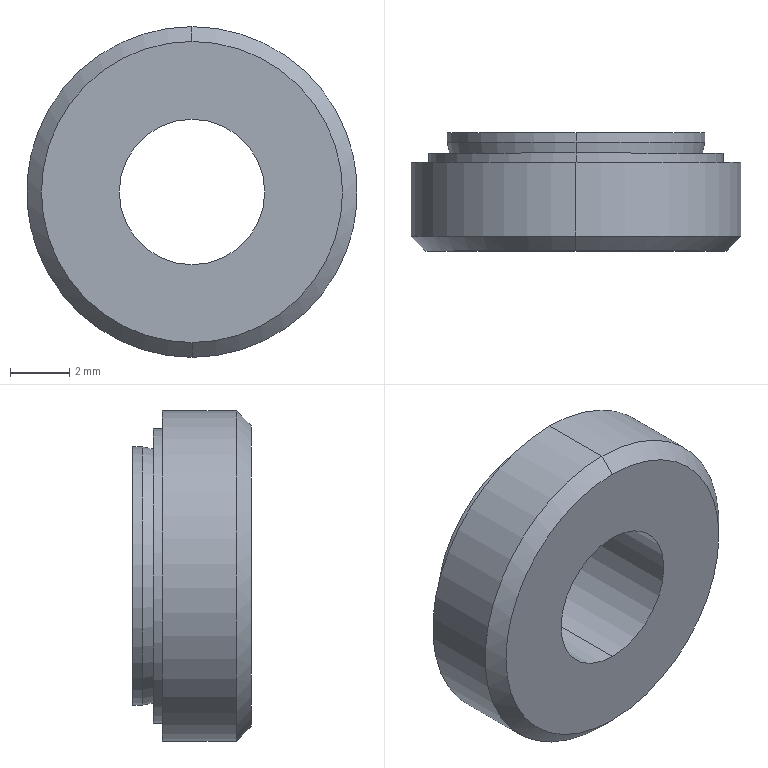Part | NX | features solid 2 | 1 solid | 18 faces | box 11.18 x 4 x 11.18 mm | volume 276.924 mm3 | cylinder 8 | cone 6 | plane 4 | commonest cylinder face diameters 4.917 x2 8.73 x2 9.955 x2 11.18 x2
STEP:
#1=CARTESIAN_POINT('',(-24.5,-9.,-1048.59));
#2=VERTEX_POINT('',#1);
#3=CARTESIAN_POINT('',(-24.5,-6.5,-1048.59));
#4=VERTEX_POINT('',#3);
#5=CARTESIAN_POINT('',(-24.5,-9.,-1048.59));
#6=DIRECTION('',(0.,1.,0.));
#7=VECTOR('',#6,1000.);
#8=LINE('',#5,#7);
#9=EDGE_CURVE('',#2,#4,#8,.T.);
#10=ORIENTED_EDGE('',*,*,#9,.T.);
#11=CARTESIAN_POINT('',(-24.5,-6.5,-1037.41));
#12=VERTEX_POINT('',#11);
#13=CARTESIAN_POINT('',(-24.5,-6.5,-1043.));
#14=DIRECTION('',(0.,-1.,0.));
#15=DIRECTION('',(0.,0.,-1.));
#16=AXIS2_PLACEMENT_3D('',#13,#14,#15);
#17=CIRCLE('',#16,5.59);
#18=EDGE_CURVE('',#4,#12,#17,.T.);
#19=ORIENTED_EDGE('',*,*,#18,.T.);
#20=CARTESIAN_POINT('',(-24.5,-9.,-1037.41));
#21=VERTEX_POINT('',#20);
#22=CARTESIAN_POINT('',(-24.5,-6.5,-1037.41));
#23=DIRECTION('',(0.,-1.,0.));
#24=VECTOR('',#23,1000.);
#25=LINE('',#22,#24);
#26=EDGE_CURVE('',#12,#21,#25,.T.);
#27=ORIENTED_EDGE('',*,*,#26,.T.);
#28=CARTESIAN_POINT('',(-24.5,-9.,-1043.));
#29=DIRECTION('',(0.,1.,0.));
#30=DIRECTION('',(0.,0.,1.));
#31=AXIS2_PLACEMENT_3D('',#28,#29,#30);
#32=CIRCLE('',#31,5.59);
#33=EDGE_CURVE('',#21,#2,#32,.T.);
#34=ORIENTED_EDGE('',*,*,#33,.T.);
#35=EDGE_LOOP('',(#10,#19,#27,#34));
#36=FACE_BOUND('',#35,.T.);
#37=CARTESIAN_POINT('',(-24.5,-8.752,-1043.));
#38=DIRECTION('',(0.,1.,0.));
#39=DIRECTION('',(0.,0.,1.));
#40=AXIS2_PLACEMENT_3D('',#37,#38,#39);
#41=CYLINDRICAL_SURFACE('',#40,5.59);
#42=ADVANCED_FACE('',(#36),#41,.T.);
#43=CARTESIAN_POINT('',(-24.5,-9.5,-1037.91));
#44=VERTEX_POINT('',#43);
#45=CARTESIAN_POINT('',(-24.5,-9.,-1037.41));
#46=DIRECTION('',(0.,-0.7071,-0.7071));
#47=VECTOR('',#46,1000.);
#48=LINE('',#45,#47);
#49=EDGE_CURVE('',#21,#44,#48,.T.);
#50=ORIENTED_EDGE('',*,*,#49,.T.);
#51=CARTESIAN_POINT('',(-24.5,-9.5,-1048.09));
#52=VERTEX_POINT('',#51);
#53=CARTESIAN_POINT('',(-24.5,-9.5,-1043.));
#54=DIRECTION('',(0.,1.,0.));
#55=DIRECTION('',(0.,0.,1.));
#56=AXIS2_PLACEMENT_3D('',#53,#54,#55);
#57=CIRCLE('',#56,5.09);
#58=EDGE_CURVE('',#44,#52,#57,.T.);
#59=ORIENTED_EDGE('',*,*,#58,.T.);
#60=CARTESIAN_POINT('',(-24.5,-9.,-1048.59));
#61=DIRECTION('',(0.,-0.7071,0.7071));
#62=VECTOR('',#61,1000.);
#63=LINE('',#60,#62);
#64=EDGE_CURVE('',#52,#2,#63,.F.);
#65=ORIENTED_EDGE('',*,*,#64,.T.);
#66=ORIENTED_EDGE('',*,*,#33,.F.);
#67=EDGE_LOOP('',(#50,#59,#65,#66));
#68=FACE_BOUND('',#67,.T.);
#69=CARTESIAN_POINT('',(-24.5,-9.25,-1043.));
#70=DIRECTION('',(0.,1.,0.));
#71=DIRECTION('',(0.,0.,1.));
#72=AXIS2_PLACEMENT_3D('',#69,#70,#71);
#73=CONICAL_SURFACE('',#72,5.34,0.7854);
#74=ADVANCED_FACE('',(#68),#73,.T.);
#75=ORIENTED_EDGE('',*,*,#64,.F.);
#76=CARTESIAN_POINT('',(-24.5,-9.5,-1043.));
#77=DIRECTION('',(0.,1.,0.));
#78=DIRECTION('',(0.,0.,-1.));
#79=AXIS2_PLACEMENT_3D('',#76,#77,#78);
#80=CIRCLE('',#79,5.09);
#81=EDGE_CURVE('',#52,#44,#80,.T.);
#82=ORIENTED_EDGE('',*,*,#81,.T.);
#83=ORIENTED_EDGE('',*,*,#49,.F.);
#84=CARTESIAN_POINT('',(-24.5,-9.,-1043.));
#85=DIRECTION('',(0.,1.,0.));
#86=DIRECTION('',(0.,0.,-1.));
#87=AXIS2_PLACEMENT_3D('',#84,#85,#86);
#88=CIRCLE('',#87,5.59);
#89=EDGE_CURVE('',#2,#21,#88,.T.);
#90=ORIENTED_EDGE('',*,*,#89,.F.);
#91=EDGE_LOOP('',(#75,#82,#83,#90));
#92=FACE_BOUND('',#91,.T.);
#93=CARTESIAN_POINT('',(-24.5,-9.25,-1043.));
#94=DIRECTION('',(0.,1.,0.));
#95=DIRECTION('',(0.,0.,1.));
#96=AXIS2_PLACEMENT_3D('',#93,#94,#95);
#97=CONICAL_SURFACE('',#96,5.34,0.7854);
#98=ADVANCED_FACE('',(#92),#97,.T.);
#99=ORIENTED_EDGE('',*,*,#26,.F.);
#100=CARTESIAN_POINT('',(-24.5,-6.5,-1043.));
#101=DIRECTION('',(0.,-1.,0.));
#102=DIRECTION('',(0.,0.,1.));
#103=AXIS2_PLACEMENT_3D('',#100,#101,#102);
#104=CIRCLE('',#103,5.59);
#105=EDGE_CURVE('',#12,#4,#104,.T.);
#106=ORIENTED_EDGE('',*,*,#105,.T.);
#107=ORIENTED_EDGE('',*,*,#9,.F.);
#108=ORIENTED_EDGE('',*,*,#89,.T.);
#109=EDGE_LOOP('',(#99,#106,#107,#108));
#110=FACE_BOUND('',#109,.T.);
#111=CARTESIAN_POINT('',(-24.5,-8.752,-1043.));
#112=DIRECTION('',(0.,1.,0.));
#113=DIRECTION('',(0.,0.,-1.));
#114=AXIS2_PLACEMENT_3D('',#111,#112,#113);
#115=CYLINDRICAL_SURFACE('',#114,5.59);
#116=ADVANCED_FACE('',(#110),#115,.T.);
#117=ORIENTED_EDGE('',*,*,#18,.F.);
#118=ORIENTED_EDGE('',*,*,#105,.F.);
#119=EDGE_LOOP('',(#117,#118));
#120=FACE_BOUND('',#119,.T.);
#121=CARTESIAN_POINT('',(-24.5,-6.5,-1038.023));
#122=VERTEX_POINT('',#121);
#123=CARTESIAN_POINT('',(-24.5,-6.5,-1047.977));
#124=VERTEX_POINT('',#123);
#125=CARTESIAN_POINT('',(-24.5,-6.5,-1043.));
#126=DIRECTION('',(0.,1.,0.));
#127=DIRECTION('',(0.,0.,1.));
#128=AXIS2_PLACEMENT_3D('',#125,#126,#127);
#129=CIRCLE('',#128,4.978);
#130=EDGE_CURVE('',#122,#124,#129,.T.);
#131=ORIENTED_EDGE('',*,*,#130,.F.);
#132=CARTESIAN_POINT('',(-24.5,-6.5,-1043.));
#133=DIRECTION('',(0.,1.,0.));
#134=DIRECTION('',(0.,0.,-1.));
#135=AXIS2_PLACEMENT_3D('',#132,#133,#134);
#136=CIRCLE('',#135,4.978);
#137=EDGE_CURVE('',#124,#122,#136,.T.);
#138=ORIENTED_EDGE('',*,*,#137,.F.);
#139=EDGE_LOOP('',(#131,#138));
#140=FACE_BOUND('',#139,.T.);
#141=CARTESIAN_POINT('',(-24.5,-6.5,-1043.));
#142=DIRECTION('',(0.,-1.,0.));
#143=DIRECTION('',(0.,0.,-1.));
#144=AXIS2_PLACEMENT_3D('',#141,#142,#143);
#145=PLANE('',#144);
#146=ADVANCED_FACE('',(#120,#140),#145,.F.);
#147=CARTESIAN_POINT('',(-24.5,-6.19,-1038.023));
#148=VERTEX_POINT('',#147);
#149=CARTESIAN_POINT('',(-24.5,-6.19,-1047.977));
#150=VERTEX_POINT('',#149);
#151=CARTESIAN_POINT('',(-24.5,-6.19,-1043.));
#152=DIRECTION('',(0.,-1.,0.));
#153=DIRECTION('',(0.,0.,1.));
#154=AXIS2_PLACEMENT_3D('',#151,#152,#153);
#155=CIRCLE('',#154,4.978);
#156=EDGE_CURVE('',#148,#150,#155,.T.);
#157=ORIENTED_EDGE('',*,*,#156,.T.);
#158=CARTESIAN_POINT('',(-24.5,-6.19,-1047.977));
#159=DIRECTION('',(0.,-1.,0.));
#160=VECTOR('',#159,1000.);
#161=LINE('',#158,#160);
#162=EDGE_CURVE('',#150,#124,#161,.T.);
#163=ORIENTED_EDGE('',*,*,#162,.T.);
#164=ORIENTED_EDGE('',*,*,#137,.T.);
#165=CARTESIAN_POINT('',(-24.5,-6.5,-1038.023));
#166=DIRECTION('',(0.,1.,0.));
#167=VECTOR('',#166,1000.);
#168=LINE('',#165,#167);
#169=EDGE_CURVE('',#122,#148,#168,.T.);
#170=ORIENTED_EDGE('',*,*,#169,.T.);
#171=EDGE_LOOP('',(#157,#163,#164,#170));
#172=FACE_BOUND('',#171,.T.);
#173=CARTESIAN_POINT('',(-24.5,-6.535,-1043.));
#174=DIRECTION('',(0.,-1.,0.));
#175=DIRECTION('',(0.,0.,1.));
#176=AXIS2_PLACEMENT_3D('',#173,#174,#175);
#177=CYLINDRICAL_SURFACE('',#176,4.978);
#178=ADVANCED_FACE('',(#172),#177,.T.);
#179=ORIENTED_EDGE('',*,*,#130,.T.);
#180=ORIENTED_EDGE('',*,*,#162,.F.);
#181=CARTESIAN_POINT('',(-24.5,-6.19,-1043.));
#182=DIRECTION('',(0.,-1.,0.));
#183=DIRECTION('',(0.,0.,-1.));
#184=AXIS2_PLACEMENT_3D('',#181,#182,#183);
#185=CIRCLE('',#184,4.978);
#186=EDGE_CURVE('',#150,#148,#185,.T.);
#187=ORIENTED_EDGE('',*,*,#186,.T.);
#188=ORIENTED_EDGE('',*,*,#169,.F.);
#189=EDGE_LOOP('',(#179,#180,#187,#188));
#190=FACE_BOUND('',#189,.T.);
#191=CARTESIAN_POINT('',(-24.5,-6.535,-1043.));
#192=DIRECTION('',(0.,-1.,0.));
#193=DIRECTION('',(0.,0.,-1.));
#194=AXIS2_PLACEMENT_3D('',#191,#192,#193);
#195=CYLINDRICAL_SURFACE('',#194,4.978);
#196=ADVANCED_FACE('',(#190),#195,.T.);
#197=ORIENTED_EDGE('',*,*,#156,.F.);
#198=ORIENTED_EDGE('',*,*,#186,.F.);
#199=EDGE_LOOP('',(#197,#198));
#200=FACE_BOUND('',#199,.T.);
#201=CARTESIAN_POINT('',(-24.5,-6.19,-1047.292));
#202=VERTEX_POINT('',#201);
#203=CARTESIAN_POINT('',(-24.5,-6.19,-1038.708));
#204=VERTEX_POINT('',#203);
#205=CARTESIAN_POINT('',(-24.5,-6.19,-1043.));
#206=DIRECTION('',(0.,1.,0.));
#207=DIRECTION('',(0.,0.,-1.));
#208=AXIS2_PLACEMENT_3D('',#205,#206,#207);
#209=CIRCLE('',#208,4.292);
#210=EDGE_CURVE('',#202,#204,#209,.T.);
#211=ORIENTED_EDGE('',*,*,#210,.F.);
#212=CARTESIAN_POINT('',(-24.5,-6.19,-1043.));
#213=DIRECTION('',(0.,1.,0.));
#214=DIRECTION('',(0.,0.,1.));
#215=AXIS2_PLACEMENT_3D('',#212,#213,#214);
#216=CIRCLE('',#215,4.292);
#217=EDGE_CURVE('',#204,#202,#216,.T.);
#218=ORIENTED_EDGE('',*,*,#217,.F.);
#219=EDGE_LOOP('',(#211,#218));
#220=FACE_BOUND('',#219,.T.);
#221=CARTESIAN_POINT('',(-24.5,-6.19,-1043.));
#222=DIRECTION('',(0.,-1.,0.));
#223=DIRECTION('',(0.,0.,-1.));
#224=AXIS2_PLACEMENT_3D('',#221,#222,#223);
#225=PLANE('',#224);
#226=ADVANCED_FACE('',(#200,#220),#225,.F.);
#227=ORIENTED_EDGE('',*,*,#217,.T.);
#228=CARTESIAN_POINT('',(-24.5,-5.818,-1047.365));
#229=VERTEX_POINT('',#228);
#230=CARTESIAN_POINT('',(-24.5,-6.19,-1047.292));
#231=DIRECTION('',(0.,0.9814,-0.1922));
#232=VECTOR('',#231,1000.);
#233=LINE('',#230,#232);
#234=EDGE_CURVE('',#202,#229,#233,.T.);
#235=ORIENTED_EDGE('',*,*,#234,.T.);
#236=CARTESIAN_POINT('',(-24.5,-5.818,-1038.635));
#237=VERTEX_POINT('',#236);
#238=CARTESIAN_POINT('',(-24.5,-5.818,-1043.));
#239=DIRECTION('',(0.,1.,0.));
#240=DIRECTION('',(0.,0.,1.));
#241=AXIS2_PLACEMENT_3D('',#238,#239,#240);
#242=CIRCLE('',#241,4.365);
#243=EDGE_CURVE('',#237,#229,#242,.T.);
#244=ORIENTED_EDGE('',*,*,#243,.F.);
#245=CARTESIAN_POINT('',(-24.5,-5.818,-1038.635));
#246=DIRECTION('',(0.,-0.9814,-0.1922));
#247=VECTOR('',#246,1000.);
#248=LINE('',#245,#247);
#249=EDGE_CURVE('',#237,#204,#248,.T.);
#250=ORIENTED_EDGE('',*,*,#249,.T.);
#251=EDGE_LOOP('',(#227,#235,#244,#250));
#252=FACE_BOUND('',#251,.T.);
#253=CARTESIAN_POINT('',(-24.5,-6.004,-1043.));
#254=DIRECTION('',(0.,1.,0.));
#255=DIRECTION('',(0.,0.,1.));
#256=AXIS2_PLACEMENT_3D('',#253,#254,#255);
#257=CONICAL_SURFACE('',#256,4.329,0.1934);
#258=ADVANCED_FACE('',(#252),#257,.T.);
#259=CARTESIAN_POINT('',(-24.5,-5.818,-1043.));
#260=DIRECTION('',(0.,1.,0.));
#261=DIRECTION('',(0.,0.,-1.));
#262=AXIS2_PLACEMENT_3D('',#259,#260,#261);
#263=CIRCLE('',#262,4.365);
#264=EDGE_CURVE('',#229,#237,#263,.T.);
#265=ORIENTED_EDGE('',*,*,#264,.F.);
#266=ORIENTED_EDGE('',*,*,#234,.F.);
#267=ORIENTED_EDGE('',*,*,#210,.T.);
#268=ORIENTED_EDGE('',*,*,#249,.F.);
#269=EDGE_LOOP('',(#265,#266,#267,#268));
#270=FACE_BOUND('',#269,.T.);
#271=CARTESIAN_POINT('',(-24.5,-6.004,-1043.));
#272=DIRECTION('',(0.,1.,0.));
#273=DIRECTION('',(0.,0.,-1.));
#274=AXIS2_PLACEMENT_3D('',#271,#272,#273);
#275=CONICAL_SURFACE('',#274,4.329,0.1934);
#276=ADVANCED_FACE('',(#270),#275,.T.);
#277=CARTESIAN_POINT('',(-24.5,-5.5,-1038.635));
#278=VERTEX_POINT('',#277);
#279=CARTESIAN_POINT('',(-24.5,-5.5,-1047.365));
#280=VERTEX_POINT('',#279);
#281=CARTESIAN_POINT('',(-24.5,-5.5,-1043.));
#282=DIRECTION('',(0.,-1.,0.));
#283=DIRECTION('',(0.,0.,1.));
#284=AXIS2_PLACEMENT_3D('',#281,#282,#283);
#285=CIRCLE('',#284,4.365);
#286=EDGE_CURVE('',#278,#280,#285,.T.);
#287=ORIENTED_EDGE('',*,*,#286,.T.);
#288=CARTESIAN_POINT('',(-24.5,-5.818,-1047.365));
#289=DIRECTION('',(0.,1.,-0.000001356));
#290=VECTOR('',#289,1000.);
#291=LINE('',#288,#290);
#292=EDGE_CURVE('',#229,#280,#291,.T.);
#293=ORIENTED_EDGE('',*,*,#292,.F.);
#294=ORIENTED_EDGE('',*,*,#264,.T.);
#295=CARTESIAN_POINT('',(-24.5,-5.5,-1038.635));
#296=DIRECTION('',(0.,-1.,-0.000001356));
#297=VECTOR('',#296,1000.);
#298=LINE('',#295,#297);
#299=EDGE_CURVE('',#278,#237,#298,.T.);
#300=ORIENTED_EDGE('',*,*,#299,.F.);
#301=EDGE_LOOP('',(#287,#293,#294,#300));
#302=FACE_BOUND('',#301,.T.);
#303=CARTESIAN_POINT('',(-24.5,-5.659,-1043.));
#304=DIRECTION('',(0.,1.,0.));
#305=DIRECTION('',(0.,0.,-1.));
#306=AXIS2_PLACEMENT_3D('',#303,#304,#305);
#307=CYLINDRICAL_SURFACE('',#306,4.365);
#308=ADVANCED_FACE('',(#302),#307,.T.);
#309=ORIENTED_EDGE('',*,*,#243,.T.);
#310=ORIENTED_EDGE('',*,*,#292,.T.);
#311=CARTESIAN_POINT('',(-24.5,-5.5,-1043.));
#312=DIRECTION('',(0.,-1.,0.));
#313=DIRECTION('',(0.,0.,-1.));
#314=AXIS2_PLACEMENT_3D('',#311,#312,#313);
#315=CIRCLE('',#314,4.365);
#316=EDGE_CURVE('',#280,#278,#315,.T.);
#317=ORIENTED_EDGE('',*,*,#316,.T.);
#318=ORIENTED_EDGE('',*,*,#299,.T.);
#319=EDGE_LOOP('',(#309,#310,#317,#318));
#320=FACE_BOUND('',#319,.T.);
#321=CARTESIAN_POINT('',(-24.5,-5.659,-1043.));
#322=DIRECTION('',(0.,1.,0.));
#323=DIRECTION('',(0.,0.,1.));
#324=AXIS2_PLACEMENT_3D('',#321,#322,#323);
#325=CYLINDRICAL_SURFACE('',#324,4.365);
#326=ADVANCED_FACE('',(#320),#325,.T.);
#327=ORIENTED_EDGE('',*,*,#316,.F.);
#328=ORIENTED_EDGE('',*,*,#286,.F.);
#329=EDGE_LOOP('',(#327,#328));
#330=FACE_BOUND('',#329,.T.);
#331=CARTESIAN_POINT('',(-24.5,-5.5,-1046.));
#332=VERTEX_POINT('',#331);
#333=CARTESIAN_POINT('',(-24.5,-5.5,-1040.));
#334=VERTEX_POINT('',#333);
#335=CARTESIAN_POINT('',(-24.5,-5.5,-1043.));
#336=DIRECTION('',(0.,-1.,0.));
#337=DIRECTION('',(0.,0.,-1.));
#338=AXIS2_PLACEMENT_3D('',#335,#336,#337);
#339=CIRCLE('',#338,3.);
#340=EDGE_CURVE('',#332,#334,#339,.F.);
#341=ORIENTED_EDGE('',*,*,#340,.F.);
#342=CARTESIAN_POINT('',(-24.5,-5.5,-1043.));
#343=DIRECTION('',(0.,-1.,0.));
#344=DIRECTION('',(0.,0.,-1.));
#345=AXIS2_PLACEMENT_3D('',#342,#343,#344);
#346=CIRCLE('',#345,3.);
#347=EDGE_CURVE('',#334,#332,#346,.F.);
#348=ORIENTED_EDGE('',*,*,#347,.F.);
#349=EDGE_LOOP('',(#341,#348));
#350=FACE_BOUND('',#349,.T.);
#351=CARTESIAN_POINT('',(-24.5,-5.5,-1043.));
#352=DIRECTION('',(0.,-1.,0.));
#353=DIRECTION('',(0.,0.,-1.));
#354=AXIS2_PLACEMENT_3D('',#351,#352,#353);
#355=PLANE('',#354);
#356=ADVANCED_FACE('',(#330,#350),#355,.F.);
#357=ORIENTED_EDGE('',*,*,#347,.T.);
#358=CARTESIAN_POINT('',(-24.5,-6.042,-1045.458));
#359=VERTEX_POINT('',#358);
#360=CARTESIAN_POINT('',(-24.5,-5.5,-1046.));
#361=DIRECTION('',(0.,-0.7071,0.7071));
#362=VECTOR('',#361,1000.);
#363=LINE('',#360,#362);
#364=EDGE_CURVE('',#332,#359,#363,.T.);
#365=ORIENTED_EDGE('',*,*,#364,.T.);
#366=CARTESIAN_POINT('',(-24.5,-6.042,-1040.542));
#367=VERTEX_POINT('',#366);
#368=CARTESIAN_POINT('',(-24.5,-6.042,-1043.));
#369=DIRECTION('',(0.,1.,0.));
#370=DIRECTION('',(0.,0.,1.));
#371=AXIS2_PLACEMENT_3D('',#368,#369,#370);
#372=CIRCLE('',#371,2.458);
#373=EDGE_CURVE('',#367,#359,#372,.T.);
#374=ORIENTED_EDGE('',*,*,#373,.F.);
#375=CARTESIAN_POINT('',(-24.5,-6.042,-1040.542));
#376=DIRECTION('',(0.,0.7071,0.7071));
#377=VECTOR('',#376,1000.);
#378=LINE('',#375,#377);
#379=EDGE_CURVE('',#367,#334,#378,.T.);
#380=ORIENTED_EDGE('',*,*,#379,.T.);
#381=EDGE_LOOP('',(#357,#365,#374,#380));
#382=FACE_BOUND('',#381,.T.);
#383=CARTESIAN_POINT('',(-24.5,-5.771,-1043.));
#384=DIRECTION('',(0.,1.,0.));
#385=DIRECTION('',(0.,0.,-1.));
#386=AXIS2_PLACEMENT_3D('',#383,#384,#385);
#387=CONICAL_SURFACE('',#386,2.729,0.7854);
#388=ADVANCED_FACE('',(#382),#387,.F.);
#389=CARTESIAN_POINT('',(-24.5,-6.042,-1043.));
#390=DIRECTION('',(0.,1.,0.));
#391=DIRECTION('',(0.,0.,1.));
#392=AXIS2_PLACEMENT_3D('',#389,#390,#391);
#393=CIRCLE('',#392,2.458);
#394=EDGE_CURVE('',#359,#367,#393,.T.);
#395=ORIENTED_EDGE('',*,*,#394,.F.);
#396=ORIENTED_EDGE('',*,*,#364,.F.);
#397=ORIENTED_EDGE('',*,*,#340,.T.);
#398=ORIENTED_EDGE('',*,*,#379,.F.);
#399=EDGE_LOOP('',(#395,#396,#397,#398));
#400=FACE_BOUND('',#399,.T.);
#401=CARTESIAN_POINT('',(-24.5,-5.771,-1043.));
#402=DIRECTION('',(0.,1.,0.));
#403=DIRECTION('',(0.,0.,1.));
#404=AXIS2_PLACEMENT_3D('',#401,#402,#403);
#405=CONICAL_SURFACE('',#404,2.729,0.7854);
#406=ADVANCED_FACE('',(#400),#405,.F.);
#407=CARTESIAN_POINT('',(-24.5,-9.5,-1045.458));
#408=VERTEX_POINT('',#407);
#409=CARTESIAN_POINT('',(-24.5,-6.042,-1045.458));
#410=DIRECTION('',(0.,-1.,-0.00000087));
#411=VECTOR('',#410,1000.);
#412=LINE('',#409,#411);
#413=EDGE_CURVE('',#359,#408,#412,.T.);
#414=ORIENTED_EDGE('',*,*,#413,.F.);
#415=ORIENTED_EDGE('',*,*,#394,.T.);
#416=CARTESIAN_POINT('',(-24.5,-9.5,-1040.542));
#417=VERTEX_POINT('',#416);
#418=CARTESIAN_POINT('',(-24.5,-9.5,-1040.542));
#419=DIRECTION('',(0.,1.,-0.00000087));
#420=VECTOR('',#419,1000.);
#421=LINE('',#418,#420);
#422=EDGE_CURVE('',#417,#367,#421,.T.);
#423=ORIENTED_EDGE('',*,*,#422,.F.);
#424=CARTESIAN_POINT('',(-24.5,-9.5,-1043.));
#425=DIRECTION('',(0.,-1.,0.));
#426=DIRECTION('',(0.,0.,1.));
#427=AXIS2_PLACEMENT_3D('',#424,#425,#426);
#428=CIRCLE('',#427,2.458);
#429=EDGE_CURVE('',#417,#408,#428,.T.);
#430=ORIENTED_EDGE('',*,*,#429,.T.);
#431=EDGE_LOOP('',(#414,#415,#423,#430));
#432=FACE_BOUND('',#431,.T.);
#433=CARTESIAN_POINT('',(-24.5,-8.23,-1043.));
#434=DIRECTION('',(0.,1.,0.));
#435=DIRECTION('',(0.,0.,1.));
#436=AXIS2_PLACEMENT_3D('',#433,#434,#435);
#437=CYLINDRICAL_SURFACE('',#436,2.458);
#438=ADVANCED_FACE('',(#432),#437,.F.);
#439=ORIENTED_EDGE('',*,*,#58,.F.);
#440=ORIENTED_EDGE('',*,*,#81,.F.);
#441=EDGE_LOOP('',(#439,#440));
#442=FACE_BOUND('',#441,.T.);
#443=CARTESIAN_POINT('',(-24.5,-9.5,-1043.));
#444=DIRECTION('',(0.,-1.,0.));
#445=DIRECTION('',(0.,0.,-1.));
#446=AXIS2_PLACEMENT_3D('',#443,#444,#445);
#447=CIRCLE('',#446,2.458);
#448=EDGE_CURVE('',#408,#417,#447,.T.);
#449=ORIENTED_EDGE('',*,*,#448,.F.);
#450=ORIENTED_EDGE('',*,*,#429,.F.);
#451=EDGE_LOOP('',(#449,#450));
#452=FACE_BOUND('',#451,.T.);
#453=CARTESIAN_POINT('',(-32.3,-9.5,-1052.237));
#454=DIRECTION('',(0.,1.,0.));
#455=DIRECTION('',(0.,0.,-1.));
#456=AXIS2_PLACEMENT_3D('',#453,#454,#455);
#457=PLANE('',#456);
#458=ADVANCED_FACE('',(#442,#452),#457,.F.);
#459=ORIENTED_EDGE('',*,*,#422,.T.);
#460=ORIENTED_EDGE('',*,*,#373,.T.);
#461=ORIENTED_EDGE('',*,*,#413,.T.);
#462=ORIENTED_EDGE('',*,*,#448,.T.);
#463=EDGE_LOOP('',(#459,#460,#461,#462));
#464=FACE_BOUND('',#463,.T.);
#465=CARTESIAN_POINT('',(-24.5,-8.23,-1043.));
#466=DIRECTION('',(0.,1.,0.));
#467=DIRECTION('',(0.,0.,-1.));
#468=AXIS2_PLACEMENT_3D('',#465,#466,#467);
#469=CYLINDRICAL_SURFACE('',#468,2.458);
#470=ADVANCED_FACE('',(#464),#469,.F.);
#471=CLOSED_SHELL('',(#42,#74,#98,#116,#146,#178,#196,#226,#258,#276,#308,#326,#356,#388,#406,#438,#458,#470));
#472=MANIFOLD_SOLID_BREP('',#471);
#473=(LENGTH_UNIT()NAMED_UNIT(*)SI_UNIT(.MILLI.,.METRE.));
#474=UNCERTAINTY_MEASURE_WITH_UNIT(LENGTH_MEASURE(0.00001),#473,'','');
#475=(NAMED_UNIT(*)PLANE_ANGLE_UNIT()SI_UNIT($,.RADIAN.));
#476=(NAMED_UNIT(*)SI_UNIT($,.STERADIAN.)SOLID_ANGLE_UNIT());
#477=(GEOMETRIC_REPRESENTATION_CONTEXT(3)GLOBAL_UNCERTAINTY_ASSIGNED_CONTEXT((#474))GLOBAL_UNIT_ASSIGNED_CONTEXT((#473,#475,#476))REPRESENTATION_CONTEXT('',''));
#478=ADVANCED_BREP_SHAPE_REPRESENTATION('',(#472),#477);